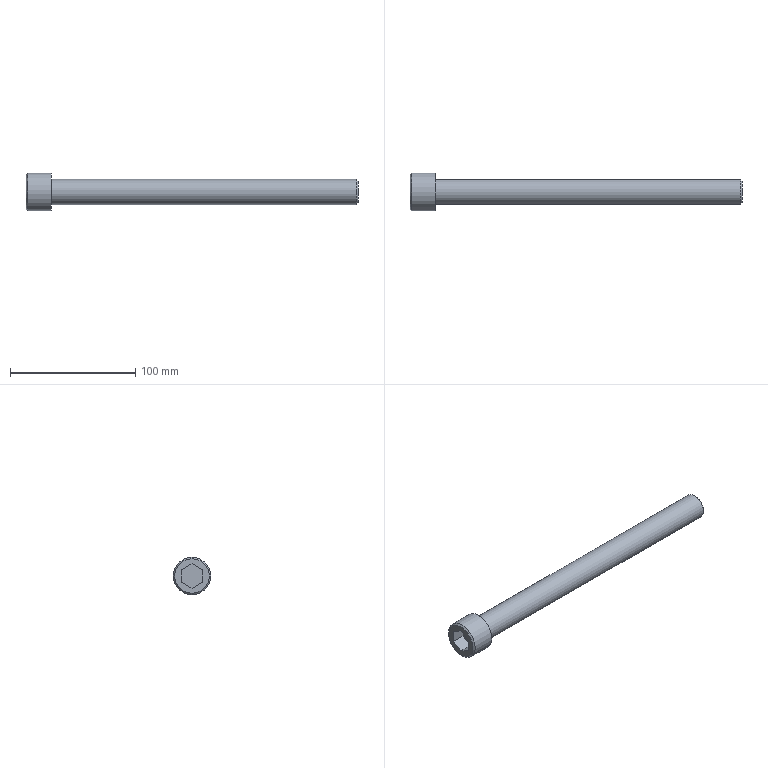Part | STEP file | solid 52 | 1 solid | 14 faces | box 265 x 30 x 30 mm | volume 88234 mm3 | plane 10 | cylinder 2 | cone 2 | commonest cylinder face diameters 20 x1 30 x1